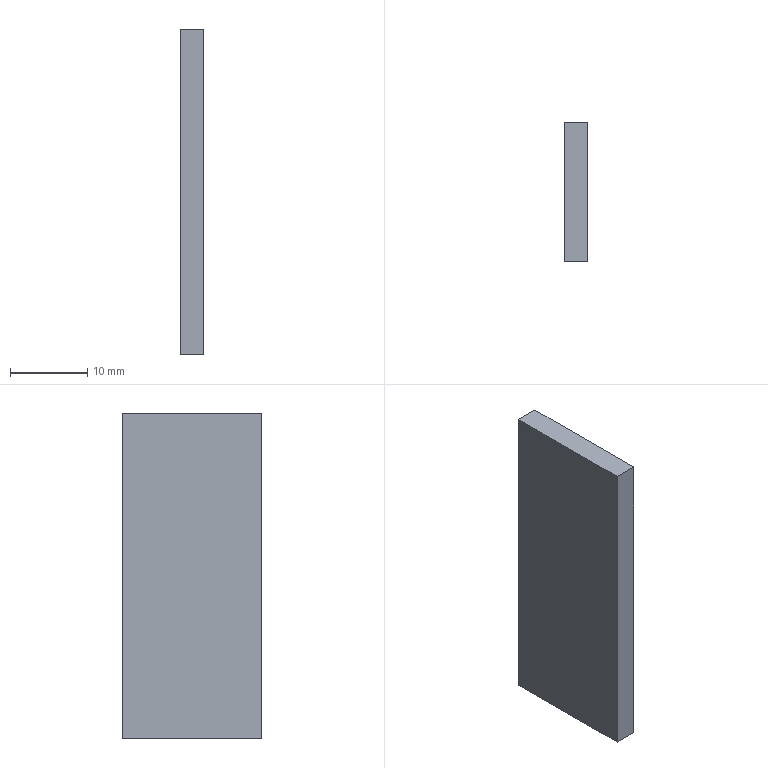Part | SolidWorks | features BaseBody 1 | 1 solid | 6 faces | box 3 x 18 x 42 mm | volume 2268 mm3 | plane 6
STEP:
#1=CARTESIAN_POINT('',(-1.5,9.,-21.));
#2=VERTEX_POINT('',#1);
#3=CARTESIAN_POINT('',(-1.5,9.,21.));
#4=VERTEX_POINT('',#3);
#5=CARTESIAN_POINT('',(-1.5,9.,-21.));
#6=DIRECTION('',(0.,0.,1.));
#7=VECTOR('',#6,1000.);
#8=LINE('',#5,#7);
#9=EDGE_CURVE('',#2,#4,#8,.T.);
#10=ORIENTED_EDGE('',*,*,#9,.F.);
#11=CARTESIAN_POINT('',(-1.5,-9.,-21.));
#12=VERTEX_POINT('',#11);
#13=CARTESIAN_POINT('',(-1.5,-9.,-21.));
#14=DIRECTION('',(0.,1.,0.));
#15=VECTOR('',#14,1000.);
#16=LINE('',#13,#15);
#17=EDGE_CURVE('',#12,#2,#16,.T.);
#18=ORIENTED_EDGE('',*,*,#17,.F.);
#19=CARTESIAN_POINT('',(-1.5,-9.,21.));
#20=VERTEX_POINT('',#19);
#21=CARTESIAN_POINT('',(-1.5,-9.,-21.));
#22=DIRECTION('',(0.,0.,-1.));
#23=VECTOR('',#22,1000.);
#24=LINE('',#21,#23);
#25=EDGE_CURVE('',#20,#12,#24,.T.);
#26=ORIENTED_EDGE('',*,*,#25,.F.);
#27=CARTESIAN_POINT('',(-1.5,-9.,21.));
#28=DIRECTION('',(0.,-1.,0.));
#29=VECTOR('',#28,1000.);
#30=LINE('',#27,#29);
#31=EDGE_CURVE('',#4,#20,#30,.T.);
#32=ORIENTED_EDGE('',*,*,#31,.F.);
#33=EDGE_LOOP('',(#10,#18,#26,#32));
#34=FACE_OUTER_BOUND('',#33,.T.);
#35=CARTESIAN_POINT('',(-1.5,-9.,-21.));
#36=DIRECTION('',(1.,0.,0.));
#37=DIRECTION('',(0.,0.,-1.));
#38=AXIS2_PLACEMENT_3D('',#35,#36,#37);
#39=PLANE('',#38);
#40=ADVANCED_FACE('',(#34),#39,.F.);
#41=CARTESIAN_POINT('',(1.5,-9.,21.));
#42=VERTEX_POINT('',#41);
#43=CARTESIAN_POINT('',(1.5,9.,21.));
#44=VERTEX_POINT('',#43);
#45=CARTESIAN_POINT('',(1.5,-9.,21.));
#46=DIRECTION('',(0.,1.,0.));
#47=VECTOR('',#46,1000.);
#48=LINE('',#45,#47);
#49=EDGE_CURVE('',#42,#44,#48,.T.);
#50=ORIENTED_EDGE('',*,*,#49,.T.);
#51=CARTESIAN_POINT('',(-1.5,9.,21.));
#52=DIRECTION('',(-1.,0.,0.));
#53=VECTOR('',#52,1000.);
#54=LINE('',#51,#53);
#55=EDGE_CURVE('',#44,#4,#54,.T.);
#56=ORIENTED_EDGE('',*,*,#55,.T.);
#57=ORIENTED_EDGE('',*,*,#31,.T.);
#58=CARTESIAN_POINT('',(-1.5,-9.,21.));
#59=DIRECTION('',(1.,0.,0.));
#60=VECTOR('',#59,1000.);
#61=LINE('',#58,#60);
#62=EDGE_CURVE('',#20,#42,#61,.T.);
#63=ORIENTED_EDGE('',*,*,#62,.T.);
#64=EDGE_LOOP('',(#50,#56,#57,#63));
#65=FACE_OUTER_BOUND('',#64,.T.);
#66=CARTESIAN_POINT('',(-1.5,-9.,21.));
#67=DIRECTION('',(0.,0.,1.));
#68=DIRECTION('',(1.,0.,0.));
#69=AXIS2_PLACEMENT_3D('',#66,#67,#68);
#70=PLANE('',#69);
#71=ADVANCED_FACE('',(#65),#70,.T.);
#72=ORIENTED_EDGE('',*,*,#55,.F.);
#73=CARTESIAN_POINT('',(1.5,9.,-21.));
#74=VERTEX_POINT('',#73);
#75=CARTESIAN_POINT('',(1.5,9.,-21.));
#76=DIRECTION('',(0.,0.,-1.));
#77=VECTOR('',#76,1000.);
#78=LINE('',#75,#77);
#79=EDGE_CURVE('',#44,#74,#78,.T.);
#80=ORIENTED_EDGE('',*,*,#79,.T.);
#81=CARTESIAN_POINT('',(-1.5,9.,-21.));
#82=DIRECTION('',(-1.,0.,0.));
#83=VECTOR('',#82,1000.);
#84=LINE('',#81,#83);
#85=EDGE_CURVE('',#74,#2,#84,.T.);
#86=ORIENTED_EDGE('',*,*,#85,.T.);
#87=ORIENTED_EDGE('',*,*,#9,.T.);
#88=EDGE_LOOP('',(#72,#80,#86,#87));
#89=FACE_OUTER_BOUND('',#88,.T.);
#90=CARTESIAN_POINT('',(-1.5,9.,-21.));
#91=DIRECTION('',(0.,1.,0.));
#92=DIRECTION('',(0.,0.,1.));
#93=AXIS2_PLACEMENT_3D('',#90,#91,#92);
#94=PLANE('',#93);
#95=ADVANCED_FACE('',(#89),#94,.T.);
#96=CARTESIAN_POINT('',(1.5,-9.,-21.));
#97=VERTEX_POINT('',#96);
#98=CARTESIAN_POINT('',(1.5,-9.,-21.));
#99=DIRECTION('',(0.,1.,0.));
#100=VECTOR('',#99,1000.);
#101=LINE('',#98,#100);
#102=EDGE_CURVE('',#97,#74,#101,.T.);
#103=ORIENTED_EDGE('',*,*,#102,.F.);
#104=CARTESIAN_POINT('',(-1.5,-9.,-21.));
#105=DIRECTION('',(1.,0.,0.));
#106=VECTOR('',#105,1000.);
#107=LINE('',#104,#106);
#108=EDGE_CURVE('',#12,#97,#107,.T.);
#109=ORIENTED_EDGE('',*,*,#108,.F.);
#110=ORIENTED_EDGE('',*,*,#17,.T.);
#111=ORIENTED_EDGE('',*,*,#85,.F.);
#112=EDGE_LOOP('',(#103,#109,#110,#111));
#113=FACE_OUTER_BOUND('',#112,.T.);
#114=CARTESIAN_POINT('',(-1.5,-9.,-21.));
#115=DIRECTION('',(0.,0.,1.));
#116=DIRECTION('',(1.,0.,0.));
#117=AXIS2_PLACEMENT_3D('',#114,#115,#116);
#118=PLANE('',#117);
#119=ADVANCED_FACE('',(#113),#118,.F.);
#120=ORIENTED_EDGE('',*,*,#62,.F.);
#121=ORIENTED_EDGE('',*,*,#25,.T.);
#122=ORIENTED_EDGE('',*,*,#108,.T.);
#123=CARTESIAN_POINT('',(1.5,-9.,-21.));
#124=DIRECTION('',(0.,0.,-1.));
#125=VECTOR('',#124,1000.);
#126=LINE('',#123,#125);
#127=EDGE_CURVE('',#42,#97,#126,.T.);
#128=ORIENTED_EDGE('',*,*,#127,.F.);
#129=EDGE_LOOP('',(#120,#121,#122,#128));
#130=FACE_OUTER_BOUND('',#129,.T.);
#131=CARTESIAN_POINT('',(-1.5,-9.,-21.));
#132=DIRECTION('',(0.,1.,0.));
#133=DIRECTION('',(0.,0.,1.));
#134=AXIS2_PLACEMENT_3D('',#131,#132,#133);
#135=PLANE('',#134);
#136=ADVANCED_FACE('',(#130),#135,.F.);
#137=ORIENTED_EDGE('',*,*,#79,.F.);
#138=ORIENTED_EDGE('',*,*,#49,.F.);
#139=ORIENTED_EDGE('',*,*,#127,.T.);
#140=ORIENTED_EDGE('',*,*,#102,.T.);
#141=EDGE_LOOP('',(#137,#138,#139,#140));
#142=FACE_OUTER_BOUND('',#141,.T.);
#143=CARTESIAN_POINT('',(1.5,-9.,-21.));
#144=DIRECTION('',(1.,0.,0.));
#145=DIRECTION('',(0.,0.,-1.));
#146=AXIS2_PLACEMENT_3D('',#143,#144,#145);
#147=PLANE('',#146);
#148=ADVANCED_FACE('',(#142),#147,.T.);
#149=CLOSED_SHELL('',(#40,#71,#95,#119,#136,#148));
#150=MANIFOLD_SOLID_BREP('',#149);
#151=CARTESIAN_POINT('',(0.,0.,0.));
#152=DIRECTION('',(0.,0.,1.));
#153=DIRECTION('',(1.,0.,0.));
#154=AXIS2_PLACEMENT_3D('',#151,#152,#153);
#155=(LENGTH_UNIT()NAMED_UNIT(*)SI_UNIT(.MILLI.,.METRE.));
#156=UNCERTAINTY_MEASURE_WITH_UNIT(LENGTH_MEASURE(0.00001),#155,'','');
#157=(NAMED_UNIT(*)PLANE_ANGLE_UNIT()SI_UNIT($,.RADIAN.));
#158=(NAMED_UNIT(*)SI_UNIT($,.STERADIAN.)SOLID_ANGLE_UNIT());
#159=(GEOMETRIC_REPRESENTATION_CONTEXT(3)GLOBAL_UNCERTAINTY_ASSIGNED_CONTEXT((#156))GLOBAL_UNIT_ASSIGNED_CONTEXT((#155,#157,#158))REPRESENTATION_CONTEXT('',''));
#160=ADVANCED_BREP_SHAPE_REPRESENTATION('',(#150,#154),#159);